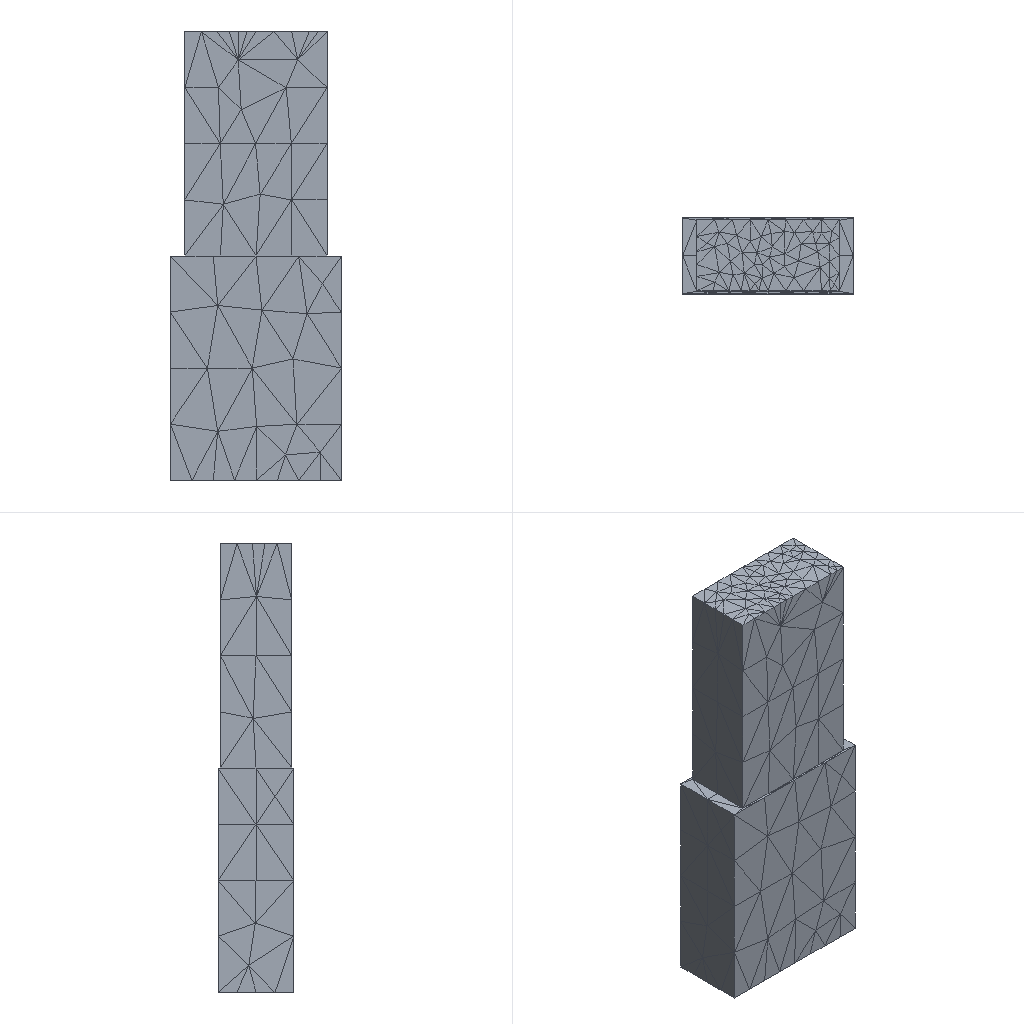Simulation study | ansys electronics desktop
Set-up summary:
category,name,step,type,value,unit,region
solver,ansys_electronics_desktop
units,length mm,,stated,model units
analysis,06_step_wg,,HFSS Modal Network,design_type=HFSS
setup,Setup1,06_step_wg,HfssDriven,frequency=10GHz; max_passes=6; max_delta_s=0.02
sweep,Sweep1,Setup1,Discrete,8GHz..12GHz n=9 step=
mesh,nodes,,,n/a (no mesh stored)
mesh,elements,,,n/a (no mesh stored)
material,vacuum,,permittivity,1
load,1,06_step_wg,wave port,,,faces 8
load,2,06_step_wg,wave port,,,faces 35
bc,PerfE,06_step_wg,perfect e,,,"faces 7, 9, 10, 11, 12, 37, 38, 39, 40"
Ansys Electronics Desktop project file, long lists of numbers shortened, first 303 of 2133 lines:
$begin 'AnsoftProject'
	Created='Fri Sep  4 17:12:09 2026'
	Product='ElectronicsDesktop'
	FileOwnedByWorkbench=false
	$begin 'Desktop'
		Version(2026, 1)
		InfrastructureVersion(1, 0)
		$begin 'FactoryHeader'
			$begin 'geometry3deditor'
				KernelVersion(2, 0)
				ProjectContainsGeometry3D='1'
			$end 'geometry3deditor'
		$end 'FactoryHeader'
	$end 'Desktop'
	UsesAdvancedFeatures=false
	PreviewImageDesignId=1
	NextUniqueID=0
	MoveBackwards=false
	$begin 'HFSSEnvironment'
		Version(1, 0)
	$end 'HFSSEnvironment'
	$begin 'PlanarEMEnvironment'
		Version(1, 0)
	$end 'PlanarEMEnvironment'
	$begin 'Q3DEnvironment'
		Version(1, 0)
	$end 'Q3DEnvironment'
	$begin '2DExtractorEnvironment'
		Version(1, 0)
	$end '2DExtractorEnvironment'
	$begin 'NexximEnvironment'
		Version(1, 0)
	$end 'NexximEnvironment'
	$begin 'NexximNetlistEnvironment'
		Version(1, 0)
	$end 'NexximNetlistEnvironment'
	$begin 'EmitEnvironment'
		Version(1, 0)
	$end 'EmitEnvironment'
	$begin 'Maxwell3DEnvironment'
		Version(1, 0)
	$end 'Maxwell3DEnvironment'
	$begin 'Maxwell2DEnvironment'
		Version(1, 0)
	$end 'Maxwell2DEnvironment'
	$begin 'RMxprtEnvironment'
		Version(1, 0)
	$end 'RMxprtEnvironment'
	$begin 'MaxCirEnvironment'
		Version(1, 0)
	$end 'MaxCirEnvironment'
	$begin 'SimplorerEnvironment'
		Version(1, 0)
	$end 'SimplorerEnvironment'
	$begin 'IcepakEnvironment'
		Version(1, 0)
	$end 'IcepakEnvironment'
	$begin 'IcepakFEAEnvironment'
		Version(1, 0)
	$end 'IcepakFEAEnvironment'
	$begin 'SchematicEnvironment'
		Version(1, 0)
	$end 'SchematicEnvironment'
	$begin 'geometry3deditor'
		Version(1, 0)
	$end 'geometry3deditor'
	ReadVersion=12
	$begin 'DesignMgrEnvironment'
		CompInstCounter=1
		GPortCounter=0
		NetCounter=0
		Alias('Ieee;Simplorer Elements\\Ieee', 'Std;Simplorer Elements\\Std', 'Basic_VHDLAMS;Simplorer Elements\\Basic Elements VHDLAMS\\Basic Elements VHDLAMS', 'Digital_Elements;Simplorer Elements\\Digital Elements\\Digital Elements', 'Transformations;Simplorer Elements\\Tools\\Transformations\\Transformations', 'HEV_VHDLAMS;Simplorer Elements\\HEV VHDLAMS\\HEV VHDLAMS', 'automotive_vda;Simplorer Elem
	$end 'DesignMgrEnvironment'
	$begin 'ProjectDatasets'
		NextUniqueID=0
		MoveBackwards=false
		DatasetType='ProjectDatasetType'
		$begin 'DatasetDefinitions'
		$end 'DatasetDefinitions'
	$end 'ProjectDatasets'
	VariableOrders[0:]
	$begin 'Definitions'
		$begin 'Materials'
			$begin 'vacuum'
				CoordinateSystemType='Cartesian'
				BulkOrSurfaceType=1
				$begin 'PhysicsTypes'
					set('Electromagnetic')
				$end 'PhysicsTypes'
				$begin 'AttachedData'
					$begin 'MatAppearanceData'
						property_data='appearance_data'
						Red=230
						Green=230
						Blue=230
						Transparency=0.95
					$end 'MatAppearanceData'
				$end 'AttachedData'
				permittivity='1'
				ModTime=1499970477
				Library='Materials'
				LibLocation='SysLibrary'
				ModSinceLib=false
			$end 'vacuum'
		$end 'Materials'
		$begin 'SurfaceMaterials'
			$begin 'Steel-oxidised-surface'
				CoordinateSystemType='Cartesian'
				BulkOrSurfaceType=2
				$begin 'PhysicsTypes'
					set('Thermal')
				$end 'PhysicsTypes'
				surface_emissivity='0.8'
				ModTime=1461288057
				Library='SurfaceMaterials'
				LibLocation='SysLibrary'
				ModSinceLib=false
			$end 'Steel-oxidised-surface'
		$end 'SurfaceMaterials'
		$begin 'Scripts'
		$end 'Scripts'
		$begin 'AnsysComponents'
			NextUniqueID=0
			MoveBackwards=false
			$begin 'AnsysComponentDefinitions'
			$end 'AnsysComponentDefinitions'
		$end 'AnsysComponents'
		$begin 'Symbols'
			$begin '06_step_wg'
				ModTime=1788513129
				Library=''
				ModSinceLib=false
				LibLocation='Project'
				HighestLevel=1
				Normalize=true
				InitialLevels(0, 1)
				$begin 'Graphics'
					Rect(0, 0, 0, 0, 0.00254, 0.00254, 0.00508, 0.00508, 0, 0, 0)
					Rect(0, 1, 0, 0, 0.0004233, 0.00254, 0.0004233, 0.0004233, 0, 0, 0)
				$end 'Graphics'
			$end '06_step_wg'
		$end 'Symbols'
		$begin 'DefInfo'
			'06_step_wg'(1002, 0, 0, 0, '', 1788513129, '', '06_step_wg', '', '', '', '', '', 'Design.bmp', '', 'Project', '', '', 1788513129, '', 0, 0)
		$end 'DefInfo'
		$begin 'Compdefs'
			$begin '06_step_wg'
				Library=''
				CircuitEnv=0
				Refbase='U'
				NumParts=1
				ModSinceLib=true
				$begin 'Properties'
					TextProp('Representation', 'SRD', '', '06_step_wg')
					TextProp('Owner', 'SRD', '', 'HFSS')
				$end 'Properties'
				CompExtID=6
				$begin 'Parameters'
					ButtonProp('CosimDefinition', 'D', '', 'Edit', 'Edit', 40501, ButtonPropClientData())
					MenuProp('CoSimulator', 'D', '', 'DefaultNetlist', 0)
				$end 'Parameters'
				$begin 'CosimDefinitions'
					$begin 'CosimDefinition'
						CosimulatorType=4
						CosimDefName='DefaultNetlist'
						IsDefinition=true
						Connect=true
						Data()
						GRef()
					$end 'CosimDefinition'
					DefaultCosim='DefaultNetlist'
				$end 'CosimDefinitions'
			$end '06_step_wg'
		$end 'Compdefs'
	$end 'Definitions'
	DesignIDServer=2
	MoveBackwards=false
	$begin 'HFSSModel'
		RepRewriteV2=true
		Name='06_step_wg'
		DesignID=0
		'Use Advanced DC Extrapolation'=false
		'Use Power S'=false
		'Export FRTM After Simulation'=false
		'Export Rays After Simulation'=false
		'Export After Simulation'=false
		'Allow Material Override'=false
		'Calculate Lossy Dielectrics'=false
		'Perform Minimal validation'=false
		$begin 'TemperatureSettings'
			IncludeTemperatureDependence=false
			EnableFeedback=false
			Temperatures(6, '22cel')
		$end 'TemperatureSettings'
		ObjsEnabledForDeformation()
		'Port Validation Settings'='Standard'
		'Save Adaptive support files'=false
		SolutionType='HFSS Modal Network'
		$begin 'DrivenOptions'
			AutoOpen=false
		$end 'DrivenOptions'
		HasTransientSetups=false
		MaterialDensity=1
		MassOfTissue=1
		VoxelSize=1
		TissueObjectList=-1
		AverageSarMethod=0
		UseAutoDCThickness=true
		HaveZwaveSupport=true
		SolveInsideThreshold=100000
		RequireBodyFaceInfo=false
		$begin 'OutputVariable'
			NextUniqueID=0
			MoveBackwards=false
		$end 'OutputVariable'
		$begin 'ModelSetup'
			$begin 'DesignDatasets'
				NextUniqueID=0
				MoveBackwards=false
				DatasetType='DesignDatasetType'
				$begin 'DatasetDefinitions'
				$end 'DatasetDefinitions'
			$end 'DesignDatasets'
			VariableOrders[0:]
			$begin 'Editor3D Doc Preferences'
				BackgroundColorVersion=1
				'Plane Background'=0
				'Need Lights'=true
				'Ambient Light'=8355711
				'Num Lights'=1
				Light0[4: 16777215, 0.75, -0.15, -0.63]
				Ver=2
			$end 'Editor3D Doc Preferences'
			SnapMode=31
			WorkingCS=1
			$begin 'GeometryCore'
				BlockVersionID=3
				DataVersion=2
				NativeKernel='PARASOLID'
				NativeKernelVersionID=26
				Units='mm'
				ModelExtents=10000
				InstanceID=-1
				$begin 'ValidationOptions'
					EntityCheckLevel='Strict'
					IgnoreUnclassifiedObjects=false
					SkipIntersectionChecks=false
				$end 'ValidationOptions'
				ContainsGeomLinkUDM=false
				$begin 'GeometryOperations'
					BlockVersionID=2
					$begin 'AnsoftRangedIDServerManager'
						$begin 'AnsoftRangedIDServer'
							IDServerObjectTypeID=0
							IDServerRangeMin=0
							IDServerRangeMax=2146483647
							NextUniqueID=65
							MoveBackwards=false
						$end 'AnsoftRangedIDServer'
						$begin 'AnsoftRangedIDServer'
							IDServerObjectTypeID=1
							IDServerRangeMin=2146483648
							IDServerRangeMax=2146485547
							NextUniqueID=2146483654
							MoveBackwards=false
						$end 'AnsoftRangedIDServer'
					$end 'AnsoftRangedIDServerManager'
					StartBackGroundFaceID=2146483648
					$begin 'CoordinateSystems'
					$end 'CoordinateSystems'
					$begin 'OperandCSs'
					$end 'OperandCSs'
					$begin 'SubModelDefinitions'
					$end 'SubModelDefinitions'
					$begin 'Groups'
					$end 'Groups'
					$begin 'UserDefinedModels'
					$end 'UserDefinedModels'
					$begin 'OperandUserDefinedModels'
					$end 'OperandUserDefinedModels'
					$begin 'ToplevelParts'
						$begin 'GeometryPart'
							$begin 'Attributes'
								Name='WR90'
								Flags=''
								Color='(230 230 230)'
								Transparency=0.8
								PartCoordinateSystem=1
								UDMId=-1
								GroupId=-1
								MaterialValue='"vacuum"'
								SurfaceMaterialValue='""'
								SolveInside=true
								ShellElement=false
								ShellElementThickness='0mm'
								ReferenceTemperature='20cel'
								IsMaterialEditable=true
								IsSurfaceMaterialEditable=true
								UseMaterialAppearance=false
								IsLightweight=false
								IsAlwaysHidden=false
							$end 'Attributes'
							$begin 'PhysicsAttributes'
Last 211 lines:
+p7r9f5z/tF/wDki/Dn/saYv/1ER/ox+zo/5LTxG/7FeE/9S2eH0UUV/kuf60H7gf8ABGn/AJuP/wC6\
Qf8AvUa/cCvw/wD+CNP/ADcf/wB0g/8Aeo1+4Ff7wfQy/wCUa/Df/usf+r/ND/B/6Zv/ACkp4kf90f8\
A9UGVkc0MNzDLb3EUU9vPFJDPBNGssM0MqlJYpYnBWSJkZgykEEMQQQa8F8DfsofstfDDwt478DfDT9\
mv4A/DzwT8UjdH4m+DvA3wc+HfhLwt8RTewXNreHx34e0Dw5b2ni4zWt5dxy/2hDceZHdSI+VdgfX/A\
BXaeJdQ8LeJbDwZrmleGfGF7oGs2nhPxJr3h+48W6H4f8S3OnXMOha5rPhW01/SpfE2lWmqPa3Fxp8W\
qabJew272yX9m0guI/xs+LnxX/a0/ZL8aeLfBEn7RvxC/am8H/8AClfAnxI+MfxH8Y/Cn4G6L4w/ZJt\
PFP7U/wADvhBqfxC8M2XwY+EmiaXq3g8/AfxX+1D44sdL8T6T4jvLOT9lWZrvUdU0+6u7Y/1Afy+fpb\
p/7I37KOk/CDUv2e9K/Zi/Z60z4BazdyX+sfA/T/gt8N7L4QatfTT211Le6l8NLbw0ui31211Z2kjSS\
2Tu0lrG5YsikL4m/ZH/AGUvGvwq8N/Anxl+zH+z14t+CHg24t7zwh8G/E3wX+G+vfCrwrd2gvBa3Xhv\
4ear4al0jQ7iIajqHlva2cTJ9um2kea+78DfFf8AwU88SeEviJqH7PPwz/bpvf2hvhV4t+Kf7IXhbQP\
23tD+Fvwj+JHxR0HTfj78Ov8Agof4++Ivhb4U6d8BfgqvgP49eL7Of9hnQtJ8Lto3gDWml1z4m3/hu8\
sdX1rTkS3+w/AnxZ+M/wAaPGPwE/Zm+Gv7fnxV1W28e6T+158YfE37Qf8AwzR8HPhL+1Z4V8J/s2az+\
yv4Ds/gB8VfhX8Z/gVL4b8LfEb/AITL9qOw1TVL64+FfhS/l0LS9LtbbQrCWaXXdTAP2b8PeHtA8JaD\
ovhbwpoej+GPDHhzS7DQ/D3hzw9plloug6DomlWsVlpej6Lo+mwRW+l6XbWUEMNvbwRxwwxQrHGiooA\
2K+Tf2Jfip4z+L/7Pth4g+ImsQeJPHXg34tftL/AbxX4qt9HsvDyeMNc/Zi/aX+Lv7N9/40fQtMxa6P\
c6zN8KW1Sa2tFjtIZtWeO1ihgWOJPrKgD4A+HP/KU39sj/ALMA/wCCaf8A60V/wVir8Jv2hP8AkT/hz\
/2UQ/8AqE/EOv3Z+HP/AClN/bI/7MA/4Jp/+tFf8FYq/CP9o0mHw58MYVY+VJ42e4YEAkyHwN4zcHIX\
IA+0SgD0POSM1jw/hK1bxT4NxMEvZUMBmcJa6808fkNSKS63jQn87Lqf5f8A7RX3s98DoJ+88t8RJfK\
PD+Db/NWPnKvcvgPYPP4puLxvLNvbWRhdS7rKZ53F3auiquDGp02UtlhyUG1gzbfJ9I0DU9ZkUWcCmI\
ywxvczyLDbxCaRoxKzscyRKUcv5auVCH5c4B+0fhb4GOlJDY2EV7POJ9weWJ4v7Svrq0jE11Esx2x2S\
2vlAGMmJQh3ytJHOzf1fmUlg8vxNbEP2EZ0p8rd47qyknpom1drRLVtI/j/AOiF4T8R8TeKPDHFdXK6\
tLh7h2tDFOpVpyhHEytNUoUXJJVYpqVScoqdNql7FvnqwT/b/wDYV/5Ny0v/ALK1+03/AOtOfGCvr6v\
kH9hX/k3LS/8AsrX7Tf8A6058YK+vq/lY/wCgAKKKKACiiigAooooAKKKKAPgD4jf8pTf2N/+zAP+Cl\
n/AK0V/wAEna8C+Jfwv+GeofEf4gX9/wDDvwLfX19428V3l7e3nhLQLm7u7u516/mubq6uZtPZ7i4km\
d3d3Ys7OWYkkmvffiN/ylN/Y3/7MA/4KWf+tFf8Ena88+IH/I+eNv8AsbvEn/p5va/xq/bJ4zF4Pw08\
GZYTFVMLKee49N05yg2v7Pi7NxauvJn734C4/HYDN8/ngcZVwc6mGpKTpVJ03JKq2k3BptX1szw//hU\
fwp/6Jj8Pf/CL8N//ACto/wCFR/Cn/omPw9/8Ivw3/wDK2vQqK/59/wC2s5/6G2K/8H1f/kz+nf8AWH\
P/APoeYz/wpr//ACZ9L/sdeEfCnhX/AIWL/wAIx4Y8PeHPt/8AwiP27+wdF03R/tn2X/hJ/s32v+z7a\
P7R5f2i48vfnZ577cbmz9s18j/ssf8AM9/9yx/7sNfXFf8AVt+zXr1sT9CnwXrYitKvWn/rHec5OUnb\
izPkryk23ZJJXeiSWyP4t8WsRiMX4g8QYjFV54mvU+qc06kpTnK2Cw0VeUm5O0UkrvRJJaI5rxnYeKd\
U8H+K9M8DeItM8IeNtR8Na7YeDvFut+HJPGOjeF/FN5pd1b+HvEWr+EYtd0tvFWmWWrSWlzcaaup6c1\
9FbPai+tDKLiP86vgl+yf+3d8MvAfj3wj4m/bg+BWt+KfGGmRa8fjb4G/Yi8T+FvjL4g+NdprHguWP4\
h/FrU/ih+2T498P+O/CV74P8Mah4c1DwzpHhzwr9i0bU7Ky8Gaz4NttD0u3h/RvxX4q8NeBPC3iXxv4\
z17SvC3g/wAG6BrPirxZ4n16+t9M0Pw54a8Padc6vruvazqV26xafpVnpdndXFxPKyxxQ27yOwVSa+P\
dG/4KN/sh6x4S+K/jWTx/418LaN8FvhjqXxo8c2fxH+AP7Q/wq8WSfCXSUnN58RvAfgL4l/CnSdd+Lf\
g8zwLbwX3hPTtbgury9tLG2ea8vbSCf+5z85PFdW/4J+/FnxDrNp8ete/aO8A3v7bGkfFv4ffFPw/8Z\
Iv2cb+H4G6NZ/DH4RfHP4G+FfhvH+zxP8eZtYufBCeBf2l/jncTO/xG/tk694+l1ODVre2tbTTIW2H7\
Anxt8KeKbT9oHwF+018O9M/bH1rx78VfGHxS+Kfiv9mrWfFPwQ8baP8AGD4e/s8/DLxL4F0P4CaT+0V\
o2seCfD1r4Z/ZL/Z0bTZV+IWoXyXngK4utRudTOq3KL9C6B+3h8AvEHhTxZ4xXSP2nPDWmeELzw/pk2\
l/Eb9hn9t34VeNvF+reJbbxFfabonwj+G/xN/Z50jxD8cdeTTvCmv3d/Y+DNL1670qzsRd6nDZ200Es\
tO+/wCChX7KNl4D8P8AxAh8beOddtfE3jXXfhxpvgXwf8Af2hvHPx1g8d+FdHj8Q+LPCmvfs3eDfhXf\
/ELwrrekeH7mwv8AVoNU8MWbaXY6vY3d/wDZ7e/s5JwD2b9nb4MQfAL4S6J8Nxr7eLNWTX/iF488Z+L\
DpMPh+PxZ8SvjB8R/Fnxf+Kfim18PwXlynh+w1L4j+OvFN7b2Aurr7FBfR2pu7oxG4k9urhvhp8SvA3\
xh8B+GPib8NfENr4q8D+MtMj1fw9rtpDe2iXlo0ktvLHcWGp20F1pWpQXkFzb3dndwQXlldWk1rdwQ3\
EMsSdzQB8AfDn/lKb+2R/2YB/wTT/8AWiv+CsVfgV+0/rssWj+Ab86e9tptn42EUcFzCILt3bwf4ric\
+WXKJCqSYVcclARJyVj/AH1+HP8AylN/bI/7MA/4Jp/+tFf8FYq/nT+MmlXdzbeDrnWI18j/AITY20N\
nK8czShPCfjG589/JYpFAZLaIpFlgUPzrGS0Z/X/CXDZTTxWZ57j6UK2KyarlyoKaUm41sVesoQ5lzS\
lGlCN2pRim5OzSZ/mz9Pl08NxP4I5rOUOfK8s8QqkYzip87/sTL9Iwk+Vv3bXkpKKd9NzlfAfhfUPEk\
kus/Ce4Gj+KrWKO4a1ubbTP+EP1GW0nhEWl+KdFvrdiltJFazxebYS294kV/dXsIvlG1vu34c/EiXwh\
c+HT8fNnwy1ua3+zQ69e6fGfhR4n1Ka38TJu0P4nW2uXFjo10+n+Hrq7bS9cTSdSjN7FbRQ3TDzX+C9\
M8RN4Qlj1aG8tdMgs1SKR7mSO3082zvHELS5DuifZnfylC5UhthjKyKjD7F0XVNR8WeEtT1nxuvgr4f\
8Awzv7Cxi8W6h8TLfwxrOo6/ZaPe202maRFoPiC1uNO0DV0u9emvNDvtaM11Hqdkkeo+DLyFlkf7rxI\
r47iWFSeWuGGmoz/cuKqTdOStJSqz9yhTcVJqcYUoqaalKzc6en0OfHLhnizL6mUZpkH+r+b4KpCHtY\
Saw2MnF0+WdKXLGpiMXTdWlGvQlOvUhTq0pxvGSg/wB2f2Ff+TctL/7K1+03/wCtOfGCvr6vxh/ZQ8f\
Xfw3+KnwO+FnwS8PeJ/Cn7MHxF1zxn4fsfC3j7xa2vhr2X4b/ABI+Ltr4++HvhzV7PUte8HabqUng7S\
SINT8VWEEX9q6wL34eWOt3ra9X7PV/M7Ti3GScZRdmno01umu5/pCmmk07p6prZoKKKKQwooooAKKKK\
ACiiigD4A+I3/KU39jf/swD/gpZ/wCtFf8ABJ2vIPiLrPlfEHx3F9m3eX4y8Tx7vOxu2a3fLnHlHGce\
tev/ABG/5Sm/sb/9mAf8FLP/AFor/gk7XgnxL/5KP8QP+x28V/8Ap9v6/wAb/wBsfRp1vDXwaVSPMln\
mPe7X/MBHs0eDn3HvFnAdKhi+E81/srEY+Tp1peww1fnhFc0Y2xNGtGNpa3iot7N20Mn+3f8Ap1/8j/\
8A2mj+3f8Ap1/8j/8A2mufor/n9+pYb/n1/wCTS/zPmf8AiYrxk/6LH/zH5V/8wn3R+yVf/bf+Fgfuv\
K8r/hFP49+7f/wkn+wMY2frX2RXxP8Asd/81F/7lH/3Z6+2K/6rf2bUI0/oWeDEILljH/WKy1e/Fmev\
qfZ5TxHnPFmX4fiDiDGf2hm+Yc/tq3s6VLn9lOVCn+7oQp0o8tKnCPuwjfl5pXk23zXjPxj4W+Hfg/x\
X8QPHOv6Z4V8E+BfDWu+MfGPijW7qOx0bw34W8MaXda34h1/V72UhbPTLPSbG7uLiViFjit3c8A1/PJ\
8U/wBoP9ib/gpb4c+K/wAYfB/7eXwQ8E23hX4J+H/CXgDTPhtrXgb9on4z/Dr9m7xF+07+zP8AET9oD\
41/Gv4CeB/El7q3gfw54n1v4Y/B3QCniGxSz+HOiW//AAknjuK3l1PWfDGh/wBIFFf3Keifzrav+0n4\
D8WXGs63df8ABRzw94/+E37KHxM/Z3+Ln7N3/BSP4ifD74Z/E74F2P7Qvxl+H/7ZXwb+LnwR+OXiL9l\
/RPh98Pdf+Gmi/BueyW51NdT8HNpOqfHvRbDUfEi65/YsN55b+zN8QdH+BP7XUn7cX7VX7Q/w7j/Z5/\
aA+I37d1l4M/aj8X2ekfBD4HeMvFHin4Of8EiPh18Odb8Lv4g1+5sPBngPVYP2Lf2kLXwXPqOuajJq2\
h6TaTx69r8+ppqWo/090UAfDP8AwTmtL2P9mBdaneWfSPiB+0Z+278XvAd5JHNFFqfwk+NX7bP7Qvxb\
+DGsWCXCKw0e9+E3jXwZdWPygGzvICo2la+5qKKAPgD4c/8AKU39sj/swD/gmn/60V/wVir+c7x14H+\
KWl2WkaTf62PGPh7RPFFnqVtrV/pWpXvjbw7YtoPiTw8LTVNF8M6fM/jyKOLU9Ll+2QPDeXF1NM1ysV\
lI19Y/0Y/Dn/lKb+2R/wBmAf8ABNP/ANaK/wCCsVfk/wCIIFns4b6NS2woRJtWMva3ADRs6P8APkSNG\
ADggu52AHj7fgevhv7QrYCrXdDE4z2cqTjOUXejJvWF1CrDnnTUotc6bUqcoO7P8yf2inH+I4Kxvgth\
XlWCznLOIqfFNDFUcVhqFSryeyyTDuWExcqc8Rgq3scXXgp0Zexq+0UMZh8XQToS+CrTU9A8PTifwxF\
aePvEaIDH461NtPHhnRJLizmt7y38KJp2+a4RJLkmWGBwbmKV7G98QNcWaxQ9n8OdWL+MYtV8QSwanr\
87NJo+rXqSm30DUTG8f2Pw9ay6gB4f0q5s2a0uIbVxPqCR28d9PdStLPJ4z4U/5Fbw1/2ANH/9N1tXe\
eGP+Rk0H/sM6X/6X2/+NftOXYWlUo4etWiqsq8Y1LS1jGUoxfMk7uU1ZJVJudS10pqLsf585dx/nnCf\
i3l+GyGUcBTyDNXlrnBKFbE4SGKqYapQqSpRp08PhqsalSbwOAo4TARqyjXeGliKcax+vv7OupXmpfG\
v9lx7kSi2g+NnjlNL+0i7N4NPuv2UvjjqnlXct1eTea8d9qF7FGIvLhgggitY4wINz/udX4MfsyXVxc\
fHX9mBJJMwxfFnxWIoAkYjjkX9mX9pG1kmDbN7SSQ2lqGDOUBhBRULPu/eev574lorD57mdJRUVCpst\
tUnd6K7d7yfWTbu9z/of4ZxMsbw/lGKlJylXoQldq17rsm7Lsr6Ky02CiiivDPdCiiigAooooAKKKKA\
PgD4jf8AKU39jf8A7MA/4KWf+tFf8Ena+Zvij4p8MW/xM+ItvceI9Bgng8deLoZ4JtX0+KaGaLxBqCS\
RSxvcBo5FdWDKQCCCCM19M/Eb/lKb+xv/ANmAf8FLP/Wiv+CTtfkt8ev+S5/Gj/srHxF/9TDWK/yZ/a\
y5FRz3w88JaVavKgqGdY6ScUne+BirO5/In0u/FXMPCrhzhDMMvymjm082xtejKNac4KChQU1KLhq23\
o76H0t/wl/hP/oaPDv/AIO9N/8Akmj/AIS/wn/0NHh3/wAHem//ACTXwjRX+GX/ABD3B/8AQxq/+AQP\
4O/4nD4l/wCiOwP/AIPxH+R+6/7FmsaTqv8Awsr+y9U07Uvs/wDwhvn/AGC9trzyfN/4SryvN+zyt5e\
7y5NucZ8tsZwa+6a/J/8A4Jgf81w/7pp/70Cv1gr/AKZv2fOXQyr6IXhHgKdR1YYf+37Skkm+fifOpu\
6Wmjlb0R/qD9HbjHE8f+DnB/FuMwdPL8Tm39oc1GlKUoQ9hmuOwy5ZS9580aKk77OTS0sYHivRLzxL4\
W8S+HNP8Ta/4Lv9f0DWdEsfGPhT+w/+Ep8JXmq6dc2Nt4m8Nf8ACT6Jqem/2/YTTpdWf9oabqFj9ptY\
/tdjd2/mQSflh4X/AGctctP2ifiD8BPhD+0p+2CnwQP7P8tr+0l4s8Q/tKfEX4t+N/Cnx91X4i/CjxN\
8JtL+FXxJ+NWp+Jbz4VeKtZ+C1t8a18aaX4XfSk0nRfHfg3WNHtfDmqX2haxX6k+M/D914t8H+K/Cth\
4p8S+Br7xN4a13w/Z+NvBkmjQ+MPB11rOl3Wm2/inwpN4j0XUtPi8S6fNcpd2LX+nX9kt1aRG6srqAS\
QSfnP4L/wCCbHijwR8EvHPwB07/AIKNft8zeBfGfgXUfBltqcTfsReGPiN4P1TW/FGh+JfEPxQ0D4qe\
Af2JtH8Q6x8XNTh03XrDU9d8Ralrs9/F491jU7pJfEjadrmnf2aftZyHwl/Zz1Lx542/aX+EGgftEft\
exfsd+EfFPwcs/C2sJ+1D8XNb+J2u/GjwpafFyx/ae+Geh/tO+L/Emp/EeP4M282ofAhbk6J4usL/AE\
3xr4K8U6BaazZ2dtr2hSfN3ws0Hx38Xvjr8Mv2W/EHxu/aavP2PfGdz+3J8f8A4AeLtH/aS+N3gz42f\
ET4OfAJP2BfhX4D03xL+0j4J8dad498afDmb4z/ALRv7Rut+G7278STzeJPCujeD767vtY0wW0tx9ja\
z/wTc17xD8Brv9nXWv8AgoD+2nL4AbWPhxdaImi+Ff8Agn54Hk8NeFfh3HryyfCu08P/AA+/YQ0nw/4\
j+FHiB9U0X/hJdD8Q6LrVvqVv4LsNNQ22kXviHT9b7rUP2FvEmr6L4En1X9uH9rq7+L/ww17xldfD/w\
DaJtdF/Yu0D4o+GvAnj/QfCOi+LPgynhjwv+x3Y/D/AFz4X3V54I8O6qYtV8EX+sx6pp8E8WtJDZ2Fv\
aAHW/sA+MvFXjP9my3HjLxF4g8X618O/jt+1/8AAOHxX4sv21bxV4m8O/s0/te/HT9nnwbr/ibWZI1f\
W/EN54P+GGhXF7fSgzXtzcS3U7vNK7t9oV5f8GfhL4Z+Bvw28O/DLwlc61qWl6E+t395rviW8t9R8T+\
K/FHizxDq3jHxv418U39nZW0F54o1vxnr+v6vqUlva2ts99rU7W9rbQmOCP1CgD4A+HP/AClN/bI/7M\
A/4Jp/+tFf8FYq/KAgz+Hp4Yk2mAyl2cqqN5c8d7IU2biWMbvjKjLoQSoIY/q/8Of+Upv7ZH/ZgH/BN\
P8A9aK/4KxV+U1ojjQb52XasiXjxnIO5RbGMng8fPG45x930wT89hMVjcN4veGywtL2tOthc6jVupNQ\
gquTyjN8rSi1UUIKUrxXtHHeaP8AIz9qkoqPgJUb5Z063Ebi9Nb/ANgJrVN2e7Ss24roj80PCn/IreG\
v+wBo/wD6bravUPAmlXGqeJdNWIlEsbiLVLmQhGEcFhLHKPkaVC3mXBghyu4oZxJsZVavP/Aenzaj4f\
8AC9vFJBAX8P6SRNdSeTAuzTIW5baSSduAFUnJ5wMkfVfw78IWEM63ekx6jf3U8Mdjd6rKCdJgiM1rL\
eGznhgWORnUJIIy8rqbURGWPful/tPAYSvQyjB42tSlSw/sKTU5LlhyuCtJSla6dmk1o2rJt6H8ucDe\
FWecZ+NmY42rl045JhuIMZWbm3Slio0sdVqKGGjZ1a6lNQhOVKPLCM23Vg05R+7P2arRoPjr+y7Mse2\
3m+K3idUbeG3XC/svftFXN0MFiw5vI25AX95hehA/eCvw8+AKqnxx/ZdRFVUX42ePFVVAVVVf2WPjsF\
VVAwAABgDgCv3Dr+ZuIazr51mNWWjnU/KKSv52Wr6s/wB/uH8MsJkuWYaNrUKUY6aLTsui7LotAooor\
xj2AooooAKKKKACiiigD4A+I3/KU39jf/swD/gpZ/60V/wSdr8lvj1/yXP40f8AZWPiL/6mGsV+tPxG\
/wCUpv7G/wD2YB/wUs/9aK/4JO1+Ln7Q2s6lF8fvjjFHc7Uj+MHxMjRfJgO1E8aa2qjLREnAA681/nR\
+0W4Hzbjjgvw5wmU4jD4epgc0xdSbxE6sIuMsIopRdKjWbd97pK3U/wAwv2nfGOWcH8CeF+JzOhXrwx\
mb4yEVQjTk044NSbl7SrSSVtrNu/QwaK89/tzVP+fr/wAgW/8A8Zo/tzVP+fr/AMgW/wD8Zr/Jj/iAH\
GX/AEM8s/8AB2K/+Yj/ABp/4jfwp/0L8x/8FYb/AOaz9ov+CYH/ADXD/umn/vQK/WCvx+/4JRX11e/8\
L7+0y+b5X/CrdnyRpt3/APCxd3+rQZzsXr6V+wNf7vfQz4fxnC30bPDfIswq0q2MwP8AbHPKjKcqb9r\
n+aVo8rnCnJ2jUineC95NK6s3/wBD30F88wnEf0WPC7OsDTqUsLjf7b5Y1VGNRez4jzelLmUJ1Iq8qb\
atN+603Z3SK/MPSP8Agph4f134N/tVfGO0+C3jjRtO/Z9/aY+D/wCzR4J0HxxqVt4J1n4pan8f/AP7J\
Piz4Q/ETxPb6xpnm/BHwJqOo/td+DGv/wC2YbjVfD/h7SJ9a1zTbHUheeG9O/TyvyH+Kn7JHxk+IHgb\
/gqT4UbwlBd6P+0n+21+zt8YvCnhO68V6Dp1r+0H+zr8OP2ZP+CcPgr45/Cm71C21GYeEbTxxZ/s+fH\
r4dSx64liPL1dr26jXRLu3vp/6gP61NzxR/wUH+Nngybxr8Itd/Zp+FVz+13oHj/9lbwZ4Z+GPhv9qD\
xJrvwF8UWP7WHi3x/ofhXWtQ/aBb9mO313wvf6H4b+EHxW1zxDpT/Da6vbaw0DTZrQXlrrdteRejeIP\
2nf2xvC2pfDH4Q6r+y3+zffftSfFy5+LHizwr8P/Df7ZnxI1D4K6Z8Cvgzp3wvtvGXxI8YfGzWv2IdN\
1zS/FQ8c/Frwhott4dsPh9qtvJ/bVneyeIIY5LqGx+AtG/YJ8JW9t8TPGdv/AMEldC0r9m/VfiN+zz4\
08L/8E47fxz+zT8Prqz+J3w48D/tG+BPi1+0nZ/DP4cfE+6+DXjbWfEfhL4t/C/w23g7xF4x0/SdU03\
4YSeJNWng12z0rTbrrPg98Cf2l/wBnj4seF/2nvB/7GfjE/DLRNf8A2pfhn8J/2Gvhl8RP2aNH+If7O\
n7PP7Qngb9gnVoItLt/EHxl0f4a6ei/tAfsdfEXXLvw7oHja5stNtfjsjaZcXb2t1ZRAH66fs3/ABrh\
/aE+EGgfE7/hGp/BerXGufEHwP4x8GXOrWniB/B/xH+EXxG8WfCL4n+FE1+wgih122034ieBvE9lDep\
Dbi7hskuDb27SGCP3OvlL9iz4VeLPg/8AAO00Dx3pS+HvGXjP4u/tM/HvxL4WGp6frcng3V/2n/2mPi\
7+0leeCLrWdHmls9Wv9Ek+K50q5ubKaeynn0eSWznntmilf6toA+APhz/ylN/bI/7MA/4Jp/8ArRX/A\
AVir8dNa8eSC1u3nt3022gsL3zIZGiuXvFaPck8Jji3xFEt7hQSu0/a/mUsqkfsX8Of+Upv7ZH/AGYB\
/wAE0/8A1or/AIKxV+Dd5F4j1i5s0uLb+y4NRdrcsEaWWNYkcyMpnkT7PiNJJBG8eZRG2wsGIH754E5\
XkmLx2dZnmuFw9fEZO8JKhLES92mpxxcq0oUm3GpPloxcW6VR0nHni6b94/yz/aUYPD18Z4FYuv7OP1\
B8SzjOo17r/wCECTcIS5ozlywbTdOfI4qS5XaS+b/hPd6Fqfha1MuqTxalpOhWph0Q6beXN3f/ANnaV\
HJJcwSowigtPMh2CSR9qqrPKkUQikk++vgVbNr1o2oeJdQuNB0plitdLtbFYxHf3Mc6rPdXU81vJb29\
t9mFrFmCMqssNyBdxxxIsn56/D+RtE0PwzqGl4srwaPpNybmEATPM9jG7mVmB85CZpQUfchSRoyuw7a\
+5Pg34rtb7w9Y6P5cUEunrHZzLG0caC78lXa5SDzCY7a6lEsi5+b7Q0yEzHMp+/4izied8J08Nh4zp1\
qdLCxhKXs5Tp0o0UqjpLk5ItyjG7n7SbUpcsotIr6OXjRw3mfiZxVwVmmEpZVnNDMsyWHtGSjmEYYmc\
U6lRSlP20Pfc6fNCmly1IRcfbKl+hXw10yx0n9of9li30+D7PC/xf8AHMzJ5s0uZW/Zg/aAjZt00jEf\
JGgxnHy9Mk1+ytfjR8Lr8an8ev2SL4FC1x8U/GjS+Wroi3C/sx/tCR3MaLJyEW4SVRknIXIZgQT+y9f\
yTX9t7aqsRKUq0ZNScm3LmTs7t630tqf6jUfZ+ypuilGlJJxSSSs1dWS069AooorI0CiiigAooooAKK\
KKAPgD4jf8pTf2N/8AswD/AIKWf+tFf8Ena/En9on/AJOB+Ov/AGWP4nf+ptrdftt8Rv8AlKb+xv8A9\
mAf8FLP/Wiv+CTtfjB+0LoWqzfH344zR2u6OX4wfEuSNvPthuR/GmtMrYaYEZUjggH1r+VPpV8OcQ8R\
cP8AClDh/IsZntbDYyvOpDB4WvipU4ugkpTjQhNxi3onJJN6J3P8dv2xFajR8NvBx1qsaSlnmPs5SUb\
/AOwR2u0eC0Vtf8I9rH/Pn/5MWv8A8fo/4R7WP+fP/wAmLX/4/X8R/wDEMPEv/o3me/8Ahpx//wAzn+\
A317Bf9BlL/wAGQ/zP1y/4JMf81+/7pX/70ev2Mr8gP+CUmnXlh/wvr7XD5Xm/8Kt8v95FJu8v/hYu/\
wD1TtjG9euOvFfr/X+kvgFleZ5N4S8J5bnGXV8pzHDfX/aYfE0alCvT58zxlSHPSqxhUhz05xnHmiua\
EoyV4tN/9UP7N+pCp9DDwanTmqkJf6xWcWmnbivPU7Nab6eoVhaP4p8MeIb/AMT6XoHiPQdc1PwRr0P\
hbxpp2j6vp+p3/hHxPceHPD/jG38OeJ7SyuHk0DXn8I+LPCuqpZ3axXDad4m0++WM217bSybtfij+zx\
f6T+xH4O/4LOa18KPhj8SfixJ8G/2vtB8QeE/ht4M0Px58XPix8W/H9/8A8Euf+CcWsBb2Hw5per+IP\
G3jbxN8QtZnvtf1p7e9vJ7vX9R13U5Hxdzj9iP7hP1R8RftA/AXwh4b+I/jHxZ8bvhF4X8I/BzxEnhD\
4u+KvEXxJ8G6J4b+FfiyTR/DfiGPwv8AEfXNS1qK18D+Im0Dxl4PvlstTltbk2fivTbkReTfWry8nrn\
7X37Jnhj4S6B8ffEv7UP7O3h74FeK76HS/C/xq1z42fDXSfhL4k1O4e9it9O0D4j3/iaPR9YvpJNN1F\
Uht7ySRmsJwqkxSbf5iv2dZrzU9S8efDz4O+IfGWh/HWH/AILdfBP4kH43/tU/sq/tE/DD4UW/xj+I/\
wDwRp8Ba38ZfiT8V/gt8bvDXgDVPFQ8SeMvC3xzj0TwXa654a1vRfEHxW+GfiSO607RtW8I3OvfZf7H\
WneJtN/4KO3On/HDXPAXi/xVY/FP/gpOvinx74H8PN4F+B/jv9oK4+E3/BIl/Aeq/BD4c634k1y48BX\
tn+z3d/FLQtb0ybxD4i1JvFXhL4iahPq9x9uvI4AD+hzw/wCIdA8WaFo/ijwrrmj+JvDPiHTbLWdA8R\
eH9TstZ0LXNH1K3ju9O1bR9X06eS31PTbi1lilhnhkeKWORXR2UgnXr4P/AOCbkElr+y9cW0UVrDoNv\
+0/+3rD4Bi05II9IT4Tx/t3/tJJ8Hl0JLQCEeHf+FWDwf8A2d5P7k2P2cw/uilfeFAHwB8Of+Upv7ZH\
/ZgH/BNP/wBaK/4KxV+Q+s6c9ncvKiYtZ3LRMoG1HYbmhIVQI8HdsHTYBgkhsfrx8Of+Upv7ZH/ZgH/\
BNP8A9aK/4KxV+U2voJtNEkTR+VHJb3CAblJgkjMKfIV4JklOBwNq+oxX3PAGawwedPAOpGNTMoJqDa\
vKNKSjJxV7txlWpq9mlzWbTlG/+SH7UjESo4rwBgvgrviiL7X/AOMda+e9vn8vzQ8Kf8it4a/7AGj/A\
Pputq9W+HurSaT4p011eVEvJRp0vkqhkb7YyrbYZyDGq362kjMhDhYjjdkq3lPhT/kVvDX/AGANH/8A\
TdbV3Hh52g1zSbnyLu4jtdQtLyWOxtLq/u/s9nMl1cvDY2UUk12y28MrbIo3kbbhEY8V+35Zrg8ErXT\
o07+nJE/gmONx2W+ONfHZbOUMbhuJ6sqbhzXb/tSS5bR1kp35ZR2nFuLum0fsP+z1L9o+Nf7LE+3Z5/\
xo8cy7M7tvmfsq/HR9u7A3Y3YzgZx0r9yK/BD9lXxFYeIvjJ+yvdaRfadqelf8Ld8Zm11DTLyHULW4l\
i/Zn/aN0q7Ed5ayNHKEn0kqVXmORZEYkrgfvfX85cR0nRzzMqTVuSo9L3smk1r6NH/SVw3iPreQ5Tie\
bndehCTbXLdtau1la7vpZW7IKKKK8Q9sKKKKACiiigAooooA+APiN/ylN/Y3/wCzAP8AgpZ/60V/wSd\
r8pPjv/yXD4y/9lW+In/qX6xX6t/Eb/lKb+xv/wBmAf8ABSz/ANaK/wCCTtflJ8d/+S4fGX/sq3xE/w\
DUv1irhu/Q/wAV/wBtN/ybDwU/7H2Yf+q+J5TRRRWp/wA75+rH/BMf/mt3/dNv/d+r9WK/Kf8A4Jj/A\
PNbv+6bf+79X6sVjP4mf9a37Mn/AJQf8Ev+7k/9a7Pwrn9G8J+FfDmo+LNY8PeGfD+hav498QW3izx1\
qmjaNp2l6j408VWfhXwz4Fs/E3iy+sbZJfEfiCLwT4L8HaNHe3jTXKaV4T0zT1kFpYWsMXQV+b/7JPx\
p/au8eW//AAUMsfizpPw88S/F74F/tJWngv4TfCvw5qv/AAjHgPw1YeIP2Cv2Ov2hfDXwbvfiafDtze\
6/Db/ET40eJbTUvGN5pcs15Lf3GpWeiadpaad4d0+T+8j7P8TfA/4K+NdB+JHhXxl8IPhd4t8L/GPV7\
TX/AIveG/E3w/8ACevaD8VNe0/w54U8H2Gt/EjR9V0mW38cavB4S8CeB9LhudTjupotO8G6VYo622nW\
cUPEeIv2Qv2TfF/wo8OfAbxZ+y/+zv4o+Bvg+7iv/CXwZ8RfBT4a638KPC19Ab1oL3w58O9S8My6Pol\
2jalqJSS2s4nU38+GHmybvmz9kz4rftWfFT9jjxV4m1TWPhn8QP2l9L/ak/bT+CMXiXUdBu/A3wtsNK\
+Dn/BQP47/ALPOj+Jo/B+iXc17e+H/AA18KfA9le2uiPqg1bxD/wAIrDpmoeKINS1O58RR/NPwX+PX7\
Sn7U3wY/wCCSfgOH9oPxb8GPiN+1j/wTuk/bQ+PHxw+GfgT4I6j4813Wfh78O/2OtO1/wAP+GtA+Kvw\
t8S+EPC1jrfxE/aytNTvTF4YkaC18Lmx0v8As5JzJGAfsz4e8PaB4S0HRfC3hTQ9H8MeGPDml2Gh+Hv\
Dnh7TLLRdB0HRNKtYrLS9H0XR9Ngit9L0u2soIYbe3gjjhhihWONFRQBsV8m/sS/FTxn8X/2fbDxB8R\
NYg8SeOvBvxa/aX+A3ivxVb6PZeHk8Ya5+zF+0v8Xf2b7/AMaPoWmYtdHudZm+FLapNbWix2kM2rPHa\
xQwLHEn1lQB8AfDn/lKb+2R/wBmAf8ABNP/ANaK/wCCsVflNDGl54dkWMboVhuJRNE0ZidlcXsTI6kh\
0cOhyOo3cjIJ/Vn4c/8AKU39sj/swD/gmn/60V/wVio8c/sp6z4HW71z4NR33xE017S8hufhr8R/Gz3\
XiTQ7QjWNXvrz4VfFLxRpV9qms+ItR1nW/Ez3mleMtae11O88R2Qg8XeENI0Y2V/zYDCVKHG3DHEv13\
2GFyaljaFalyOTqrGTwU4zjLnioOi8JdNxlfna0XNf+Mfpe/Rezf6SNPw7qZPxRh+HKvA9XMZTVfDzr\
yrU8weXczpShUpqM6KwL/dztGq6i/e03T97+c34RfCzV/E3hPwnfT77TT5vD+iyIqx7rueE6faMrqJc\
R2kEsQn8qWRmJMassLo6sft7wL8KtL0vV7DwZpuja14k8b31hZX9n4E8JaQdd8davZTak+l22taxp8B\
QeGPCh1syWcniTxDLpnhmwuNSgjvb2zhkDL9e/sz/ALEHxfm8DeDNG+Iv9p/s/wAPhHwt4e8Ma0lo3w\
78c/E3xHq+n+HLSHUdT8F6vp2ta94X8E+Fk1W2tUS41TTde1bV4L7VLZ9N8Ntb2Gq6h+qvw0+FngX4Q\
+HX8LeANFl0jS59SutY1Ce/1nXvE+va1q93FbW0mq+IvFfivU77VfEupLp9jptlDPf3lzLb6fpFlp8D\
R2NlaW8P6bmfiBjamEoYHKYfUqVOnCEqm9STjFJ26JaaN3erVtEz7Pwz+iv4beHucZnxPLLo5zxLmuI\
xGIqYrELnlF4irKrOFNP3acLz5XGCXNGMedyd7/DP7PP7Df8AwjHxJ8GftC+PLkeEfGvh+a/1zR/hz4\
Rg0yJvtut+CPEPw8J+OXi6K8v4Pif4psfCeuudNXR00uw8NXmqatptnqPibT5l1O6/Seiivz6pUqVZy\
qVZupUm7tt3bfm2f0zCEKcIwpxUIRVkkrJIKKKKgoKKKKACiiigAooooA+APiN/ylN/Y3/7MA/4KWf+\
tFf8Ena/Hn9oC5uF+PHxsVZ5go+LnxIAAlcAAeMtaAAAbgYoor+q/oq4DAY/iDiuGPwVHGwp4Og4qtT\
hUUW67u0pxkk/NH+NH7ZZJ+GfgzdJ/wDC7j9/+xfE8j+1XP8Az8T/APf6T/4qj7Vc/wDPxP8A9/pP/i\
qKK/tz/Vzh7/oQ4L/wlof/ACs/58/Zw/kX3I/XH/gljLLJ/wAL18ySSTb/AMKxxvdnxn/hYWcbjx0H5\
V+uFFFf5tePuGw+E8WuLMPhMPDC4en9Q5adOEYQjfLMHJ2jFKKvJtuy1bberP8Aq6/ZqpL6FHgskrJf\
6x/+tZnwV4B8G/gX/wAKk+Iv7WPj/wD4Sn/hIP8AhqD9oDw58dP7J/sT+yv+EH/4R/8AZY/Zp/Zo/wC\
EW+3/ANr3P/CTed/wzv8A239u8nT/AC/+Ew/s37G/9n/b74or8dP7pD9mn4F/8M7/AA68R+AP+Ep/4T\
D/AISD9oD9rH46f2t/Yn/CP/ZP+GoP2p/jJ+0v/wAIt9g/te++0f2H/wALb/sT7d5yf2n/AMI//aX2P\
T/tf2C2+SPDH7BfxP8AhH8Ff2DPCPwF/aE8FeFPjV+wz+zNpP7KunfFL4lfAPVPiZ4B+KXw0n+H3wd8\
JePINd+Enh/45+FtR8N3Oq+JfgP8M9ds2s/GcjaZNoP2OZ9Ut5ZWYooA+yP2dvgxB8AvhLonw3Gvt4s\
1ZNf+IXjzxn4sOkw+H4/FnxK+MHxH8WfF/wCKfim18PwXlynh+w1L4j+OvFN7b2Aurr7FBfR2pu7oxG\
4k9uoooA+APhz/AMpTf2yP+zAP+Caf/rRX/BWKvv8AoooAKKKKACiiigAooooAKKKKACiiigAooooA/\
9k='
	$end 'DesignInfo'
$end 'ProjectPreview'
Results summary, first 71 of 122 lines:
result,designs[0].name,1.step,,06_step_wg
result,designs[0].design_type,1.step,,HFSS
result,designs[0].solution_type,1.step,,HFSS Modal Network
result,designs[0].setups[0].name,Setup1,,Setup1
result,designs[0].setups[0].SetupType,Setup1,,HfssDriven
result,designs[0].setups[0].SolveType,Setup1,,Single
result,designs[0].setups[0].Frequency,Setup1,,10GHz
result,designs[0].setups[0].MaximumPasses,Setup1,,6
result,designs[0].setups[0].MaxDeltaS,Setup1,,0.02
result,designs[0].setups[0].IsEnabled,Setup1,,true
result,designs[0].setups[0].sweeps[0].name,Sweep1,,Sweep1
result,designs[0].setups[0].sweeps[0].RangeType,Sweep1,,LinearCount
result,designs[0].setups[0].sweeps[0].RangeStart,Sweep1,,8GHz
result,designs[0].setups[0].sweeps[0].RangeEnd,Sweep1,,12GHz
result,designs[0].setups[0].sweeps[0].RangeCount,Sweep1,,9
result,designs[0].setups[0].sweeps[0].Type,Sweep1,,Discrete
result,designs[0].setups[0].sweeps[0].IsEnabled,Sweep1,,true
result,designs[0].boundaries[0].name,PerfE,,PerfE
result,designs[0].boundaries[0].BoundType,PerfE,,Perfect E
result,designs[0].excitations[0].name,1,,1
result,designs[0].excitations[0].BoundType,1,,Wave Port
result,designs[0].excitations[0].WavePortType,1,,Modal
result,designs[0].excitations[0].NumModes,1,,1
result,designs[0].excitations[1].name,2,,2
result,designs[0].excitations[1].BoundType,2,,Wave Port
result,designs[0].excitations[1].WavePortType,2,,Modal
result,designs[0].excitations[1].NumModes,2,,1
result,designs[0].materials_assigned[0],1.step,,vacuum
result,designs[0].objects,1.step,,2
result,designs[0].model_units,1.step,,mm
result,designs[0].valid_solutions[0],1.step,,Setup1 : AdaptivePass
result,designs[0].valid_solutions[1],1.step,,Setup1 : LastAdaptive
result,designs[0].valid_solutions[2],1.step,,Setup1 : Sweep1
result,designs[0].sparams[0].freq_hz[1],1.step,,8e+09
result,designs[0].sparams[0].freq_hz[2],1.step,,8.5e+09
result,designs[0].sparams[0].freq_hz[3],1.step,,9e+09
result,designs[0].sparams[0].freq_hz[4],1.step,,9.5e+09
result,designs[0].sparams[0].freq_hz[5],1.step,,1e+10
result,designs[0].sparams[0].freq_hz[6],1.step,,1.05e+10
result,designs[0].sparams[0].freq_hz[7],1.step,,1.1e+10
result,designs[0].sparams[0].freq_hz[8],1.step,,1.15e+10
result,designs[0].sparams[0].freq_hz[9],1.step,,1.2e+10
result,designs[0].sparams[0].expr,1.step,,"dB(S(1,1))"
result,designs[0].sparams[0].min_db,1.step,,-11.95
result,designs[0].sparams[0].solution,1.step,,Setup1 : Sweep1
result,designs[0].sparams[0].value_db[1],1.step,,-0.06953
result,designs[0].sparams[0].value_db[2],1.step,,-0.2046
result,designs[0].sparams[0].value_db[3],1.step,,-4.906
result,designs[0].sparams[0].value_db[4],1.step,,-0.419
result,designs[0].sparams[0].value_db[5],1.step,,-0.7491
result,designs[0].sparams[0].value_db[6],1.step,,-11.95
result,designs[0].sparams[0].value_db[7],1.step,,-0.7936
result,designs[0].sparams[0].value_db[8],1.step,,-0.5775
result,designs[0].sparams[0].value_db[9],1.step,,-1.736
result,designs[0].sparams[0].max_db,1.step,,-0.06953
result,designs[0].sparams[1].freq_hz[1],1.step,,8e+09
result,designs[0].sparams[1].freq_hz[2],1.step,,8.5e+09
result,designs[0].sparams[1].freq_hz[3],1.step,,9e+09
result,designs[0].sparams[1].freq_hz[4],1.step,,9.5e+09
result,designs[0].sparams[1].freq_hz[5],1.step,,1e+10
result,designs[0].sparams[1].freq_hz[6],1.step,,1.05e+10
result,designs[0].sparams[1].freq_hz[7],1.step,,1.1e+10
result,designs[0].sparams[1].freq_hz[8],1.step,,1.15e+10
result,designs[0].sparams[1].freq_hz[9],1.step,,1.2e+10
result,designs[0].sparams[1].expr,1.step,,"dB(S(1,2))"
result,designs[0].sparams[1].min_db,1.step,,-17.991
result,designs[0].sparams[1].solution,1.step,,Setup1 : Sweep1
result,designs[0].sparams[1].value_db[1],1.step,,-17.991
result,designs[0].sparams[1].value_db[2],1.step,,-13.37
result,designs[0].sparams[1].value_db[3],1.step,,-1.695
result,designs[0].sparams[1].value_db[4],1.step,,-10.363